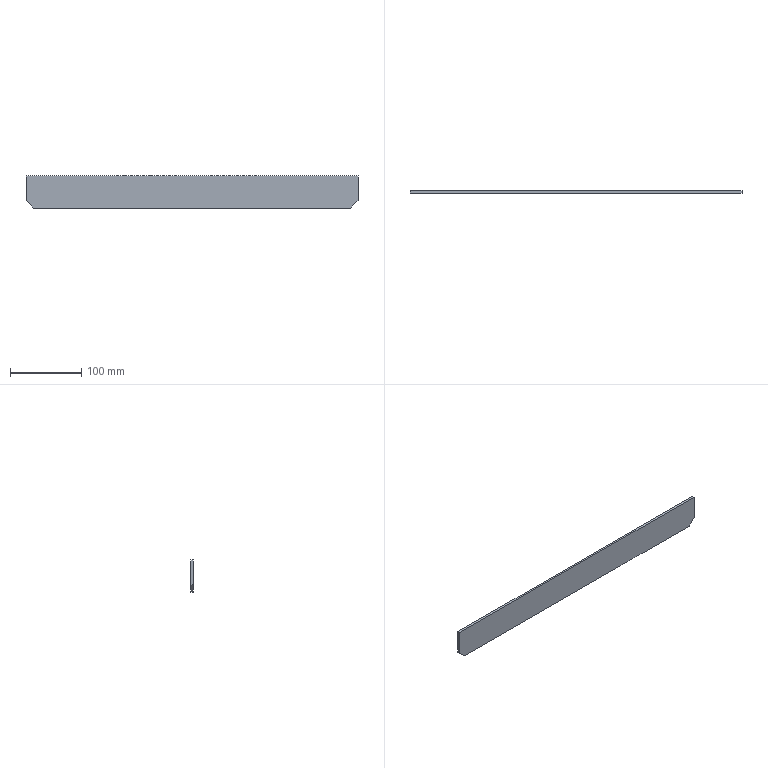Part | SolidWorks | features FlatPattern 1, SMBaseFlange 1, SheetMetal 1 | 1 solid | 8 faces | box 466 x 3.2 x 45 mm | volume 66784 mm3 | plane 8
STEP:
#1=CARTESIAN_POINT('',(466.,0.,45.));
#2=VERTEX_POINT('',#1);
#3=CARTESIAN_POINT('',(466.,0.,10.));
#4=VERTEX_POINT('',#3);
#5=CARTESIAN_POINT('',(466.,0.,10.));
#6=DIRECTION('',(0.,0.,-1.));
#7=VECTOR('',#6,1000.);
#8=LINE('',#5,#7);
#9=EDGE_CURVE('',#2,#4,#8,.T.);
#10=ORIENTED_EDGE('',*,*,#9,.F.);
#11=CARTESIAN_POINT('',(466.,-3.2,45.));
#12=VERTEX_POINT('',#11);
#13=CARTESIAN_POINT('',(466.,-3.2,45.));
#14=DIRECTION('',(0.,1.,0.));
#15=VECTOR('',#14,1000.);
#16=LINE('',#13,#15);
#17=EDGE_CURVE('',#12,#2,#16,.T.);
#18=ORIENTED_EDGE('',*,*,#17,.F.);
#19=CARTESIAN_POINT('',(466.,-3.2,10.));
#20=VERTEX_POINT('',#19);
#21=CARTESIAN_POINT('',(466.,-3.2,10.));
#22=DIRECTION('',(0.,0.,-1.));
#23=VECTOR('',#22,1000.);
#24=LINE('',#21,#23);
#25=EDGE_CURVE('',#12,#20,#24,.T.);
#26=ORIENTED_EDGE('',*,*,#25,.T.);
#27=CARTESIAN_POINT('',(466.,-3.2,10.));
#28=DIRECTION('',(0.,1.,0.));
#29=VECTOR('',#28,1000.);
#30=LINE('',#27,#29);
#31=EDGE_CURVE('',#20,#4,#30,.T.);
#32=ORIENTED_EDGE('',*,*,#31,.T.);
#33=EDGE_LOOP('',(#10,#18,#26,#32));
#34=FACE_OUTER_BOUND('',#33,.T.);
#35=CARTESIAN_POINT('',(466.,-3.2,10.));
#36=DIRECTION('',(1.,0.,0.));
#37=DIRECTION('',(0.,0.,-1.));
#38=AXIS2_PLACEMENT_3D('',#35,#36,#37);
#39=PLANE('',#38);
#40=ADVANCED_FACE('',(#34),#39,.T.);
#41=CARTESIAN_POINT('',(0.,0.,45.));
#42=VERTEX_POINT('',#41);
#43=CARTESIAN_POINT('',(0.,0.,45.));
#44=DIRECTION('',(1.,0.,0.));
#45=VECTOR('',#44,1000.);
#46=LINE('',#43,#45);
#47=EDGE_CURVE('',#42,#2,#46,.T.);
#48=ORIENTED_EDGE('',*,*,#47,.F.);
#49=CARTESIAN_POINT('',(0.,-3.2,45.));
#50=VERTEX_POINT('',#49);
#51=CARTESIAN_POINT('',(0.,-3.2,45.));
#52=DIRECTION('',(0.,1.,0.));
#53=VECTOR('',#52,1000.);
#54=LINE('',#51,#53);
#55=EDGE_CURVE('',#50,#42,#54,.T.);
#56=ORIENTED_EDGE('',*,*,#55,.F.);
#57=CARTESIAN_POINT('',(0.,-3.2,45.));
#58=DIRECTION('',(1.,0.,0.));
#59=VECTOR('',#58,1000.);
#60=LINE('',#57,#59);
#61=EDGE_CURVE('',#50,#12,#60,.T.);
#62=ORIENTED_EDGE('',*,*,#61,.T.);
#63=ORIENTED_EDGE('',*,*,#17,.T.);
#64=EDGE_LOOP('',(#48,#56,#62,#63));
#65=FACE_OUTER_BOUND('',#64,.T.);
#66=CARTESIAN_POINT('',(0.,-3.2,45.));
#67=DIRECTION('',(0.,0.,1.));
#68=DIRECTION('',(1.,0.,0.));
#69=AXIS2_PLACEMENT_3D('',#66,#67,#68);
#70=PLANE('',#69);
#71=ADVANCED_FACE('',(#65),#70,.T.);
#72=CARTESIAN_POINT('',(0.,0.,10.));
#73=VERTEX_POINT('',#72);
#74=CARTESIAN_POINT('',(0.,0.,10.));
#75=DIRECTION('',(0.,0.,1.));
#76=VECTOR('',#75,1000.);
#77=LINE('',#74,#76);
#78=EDGE_CURVE('',#73,#42,#77,.T.);
#79=ORIENTED_EDGE('',*,*,#78,.F.);
#80=CARTESIAN_POINT('',(0.,-3.2,10.));
#81=VERTEX_POINT('',#80);
#82=CARTESIAN_POINT('',(0.,-3.2,10.));
#83=DIRECTION('',(0.,1.,0.));
#84=VECTOR('',#83,1000.);
#85=LINE('',#82,#84);
#86=EDGE_CURVE('',#81,#73,#85,.T.);
#87=ORIENTED_EDGE('',*,*,#86,.F.);
#88=CARTESIAN_POINT('',(0.,-3.2,10.));
#89=DIRECTION('',(0.,0.,1.));
#90=VECTOR('',#89,1000.);
#91=LINE('',#88,#90);
#92=EDGE_CURVE('',#81,#50,#91,.T.);
#93=ORIENTED_EDGE('',*,*,#92,.T.);
#94=ORIENTED_EDGE('',*,*,#55,.T.);
#95=EDGE_LOOP('',(#79,#87,#93,#94));
#96=FACE_OUTER_BOUND('',#95,.T.);
#97=CARTESIAN_POINT('',(0.,-3.2,10.));
#98=DIRECTION('',(-1.,0.,0.));
#99=DIRECTION('',(0.,0.,1.));
#100=AXIS2_PLACEMENT_3D('',#97,#98,#99);
#101=PLANE('',#100);
#102=ADVANCED_FACE('',(#96),#101,.T.);
#103=CARTESIAN_POINT('',(10.,0.,0.));
#104=VERTEX_POINT('',#103);
#105=CARTESIAN_POINT('',(0.,0.,10.));
#106=DIRECTION('',(-0.7071,0.,0.7071));
#107=VECTOR('',#106,1000.);
#108=LINE('',#105,#107);
#109=EDGE_CURVE('',#104,#73,#108,.T.);
#110=ORIENTED_EDGE('',*,*,#109,.F.);
#111=CARTESIAN_POINT('',(10.,-3.2,0.));
#112=VERTEX_POINT('',#111);
#113=CARTESIAN_POINT('',(10.,-3.2,0.));
#114=DIRECTION('',(0.,1.,0.));
#115=VECTOR('',#114,1000.);
#116=LINE('',#113,#115);
#117=EDGE_CURVE('',#112,#104,#116,.T.);
#118=ORIENTED_EDGE('',*,*,#117,.F.);
#119=CARTESIAN_POINT('',(0.,-3.2,10.));
#120=DIRECTION('',(-0.7071,0.,0.7071));
#121=VECTOR('',#120,1000.);
#122=LINE('',#119,#121);
#123=EDGE_CURVE('',#112,#81,#122,.T.);
#124=ORIENTED_EDGE('',*,*,#123,.T.);
#125=ORIENTED_EDGE('',*,*,#86,.T.);
#126=EDGE_LOOP('',(#110,#118,#124,#125));
#127=FACE_OUTER_BOUND('',#126,.T.);
#128=CARTESIAN_POINT('',(0.,-3.2,10.));
#129=DIRECTION('',(-0.7071,0.,-0.7071));
#130=DIRECTION('',(-0.7071,0.,0.7071));
#131=AXIS2_PLACEMENT_3D('',#128,#129,#130);
#132=PLANE('',#131);
#133=ADVANCED_FACE('',(#127),#132,.T.);
#134=CARTESIAN_POINT('',(456.,0.,0.));
#135=VERTEX_POINT('',#134);
#136=CARTESIAN_POINT('',(10.,0.,0.));
#137=DIRECTION('',(-1.,0.,0.));
#138=VECTOR('',#137,1000.);
#139=LINE('',#136,#138);
#140=EDGE_CURVE('',#135,#104,#139,.T.);
#141=ORIENTED_EDGE('',*,*,#140,.F.);
#142=CARTESIAN_POINT('',(456.,-3.2,0.));
#143=VERTEX_POINT('',#142);
#144=CARTESIAN_POINT('',(456.,-3.2,0.));
#145=DIRECTION('',(0.,1.,0.));
#146=VECTOR('',#145,1000.);
#147=LINE('',#144,#146);
#148=EDGE_CURVE('',#143,#135,#147,.T.);
#149=ORIENTED_EDGE('',*,*,#148,.F.);
#150=CARTESIAN_POINT('',(10.,-3.2,0.));
#151=DIRECTION('',(-1.,0.,0.));
#152=VECTOR('',#151,1000.);
#153=LINE('',#150,#152);
#154=EDGE_CURVE('',#143,#112,#153,.T.);
#155=ORIENTED_EDGE('',*,*,#154,.T.);
#156=ORIENTED_EDGE('',*,*,#117,.T.);
#157=EDGE_LOOP('',(#141,#149,#155,#156));
#158=FACE_OUTER_BOUND('',#157,.T.);
#159=CARTESIAN_POINT('',(10.,-3.2,0.));
#160=DIRECTION('',(0.,0.,-1.));
#161=DIRECTION('',(-1.,0.,0.));
#162=AXIS2_PLACEMENT_3D('',#159,#160,#161);
#163=PLANE('',#162);
#164=ADVANCED_FACE('',(#158),#163,.T.);
#165=CARTESIAN_POINT('',(456.,0.,0.));
#166=DIRECTION('',(-0.7071,0.,-0.7071));
#167=VECTOR('',#166,1000.);
#168=LINE('',#165,#167);
#169=EDGE_CURVE('',#4,#135,#168,.T.);
#170=ORIENTED_EDGE('',*,*,#169,.F.);
#171=ORIENTED_EDGE('',*,*,#31,.F.);
#172=CARTESIAN_POINT('',(456.,-3.2,0.));
#173=DIRECTION('',(-0.7071,0.,-0.7071));
#174=VECTOR('',#173,1000.);
#175=LINE('',#172,#174);
#176=EDGE_CURVE('',#20,#143,#175,.T.);
#177=ORIENTED_EDGE('',*,*,#176,.T.);
#178=ORIENTED_EDGE('',*,*,#148,.T.);
#179=EDGE_LOOP('',(#170,#171,#177,#178));
#180=FACE_OUTER_BOUND('',#179,.T.);
#181=CARTESIAN_POINT('',(456.,-3.2,0.));
#182=DIRECTION('',(0.7071,0.,-0.7071));
#183=DIRECTION('',(-0.7071,0.,-0.7071));
#184=AXIS2_PLACEMENT_3D('',#181,#182,#183);
#185=PLANE('',#184);
#186=ADVANCED_FACE('',(#180),#185,.T.);
#187=ORIENTED_EDGE('',*,*,#25,.F.);
#188=ORIENTED_EDGE('',*,*,#61,.F.);
#189=ORIENTED_EDGE('',*,*,#92,.F.);
#190=ORIENTED_EDGE('',*,*,#123,.F.);
#191=ORIENTED_EDGE('',*,*,#154,.F.);
#192=ORIENTED_EDGE('',*,*,#176,.F.);
#193=EDGE_LOOP('',(#187,#188,#189,#190,#191,#192));
#194=FACE_OUTER_BOUND('',#193,.T.);
#195=CARTESIAN_POINT('',(0.,-3.2,0.));
#196=DIRECTION('',(0.,1.,0.));
#197=DIRECTION('',(0.,0.,1.));
#198=AXIS2_PLACEMENT_3D('',#195,#196,#197);
#199=PLANE('',#198);
#200=ADVANCED_FACE('',(#194),#199,.F.);
#201=ORIENTED_EDGE('',*,*,#9,.T.);
#202=ORIENTED_EDGE('',*,*,#169,.T.);
#203=ORIENTED_EDGE('',*,*,#140,.T.);
#204=ORIENTED_EDGE('',*,*,#109,.T.);
#205=ORIENTED_EDGE('',*,*,#78,.T.);
#206=ORIENTED_EDGE('',*,*,#47,.T.);
#207=EDGE_LOOP('',(#201,#202,#203,#204,#205,#206));
#208=FACE_OUTER_BOUND('',#207,.T.);
#209=CARTESIAN_POINT('',(0.,0.,0.));
#210=DIRECTION('',(0.,1.,0.));
#211=DIRECTION('',(0.,0.,1.));
#212=AXIS2_PLACEMENT_3D('',#209,#210,#211);
#213=PLANE('',#212);
#214=ADVANCED_FACE('',(#208),#213,.T.);
#215=CLOSED_SHELL('',(#40,#71,#102,#133,#164,#186,#200,#214));
#216=MANIFOLD_SOLID_BREP('',#215);
#217=CARTESIAN_POINT('',(0.,0.,0.));
#218=DIRECTION('',(0.,0.,1.));
#219=DIRECTION('',(1.,0.,0.));
#220=AXIS2_PLACEMENT_3D('',#217,#218,#219);
#221=(LENGTH_UNIT()NAMED_UNIT(*)SI_UNIT(.MILLI.,.METRE.));
#222=UNCERTAINTY_MEASURE_WITH_UNIT(LENGTH_MEASURE(0.00001),#221,'','');
#223=(NAMED_UNIT(*)PLANE_ANGLE_UNIT()SI_UNIT($,.RADIAN.));
#224=(NAMED_UNIT(*)SI_UNIT($,.STERADIAN.)SOLID_ANGLE_UNIT());
#225=(GEOMETRIC_REPRESENTATION_CONTEXT(3)GLOBAL_UNCERTAINTY_ASSIGNED_CONTEXT((#222))GLOBAL_UNIT_ASSIGNED_CONTEXT((#221,#223,#224))REPRESENTATION_CONTEXT('',''));
#226=ADVANCED_BREP_SHAPE_REPRESENTATION('',(#216,#220),#225);